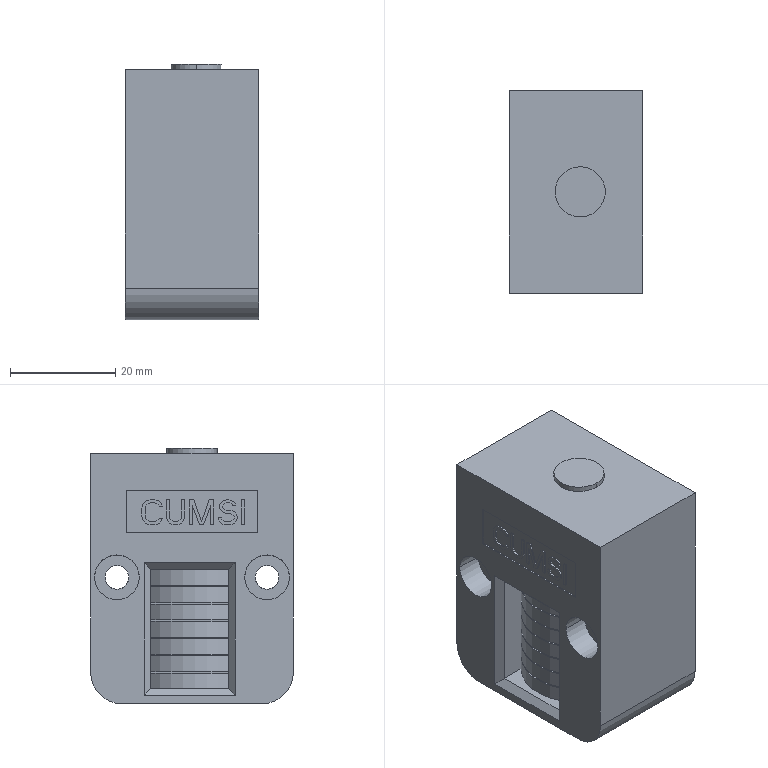Part | Creo | 1 solid | 201 faces | box 25.4 x 38.5 x 48.5 mm | volume 43458 mm3 | plane 182 | cylinder 19 | commonest cylinder face diameters 22 x7 4.5 x4 8.5 x4 9.525 x2 12 x2